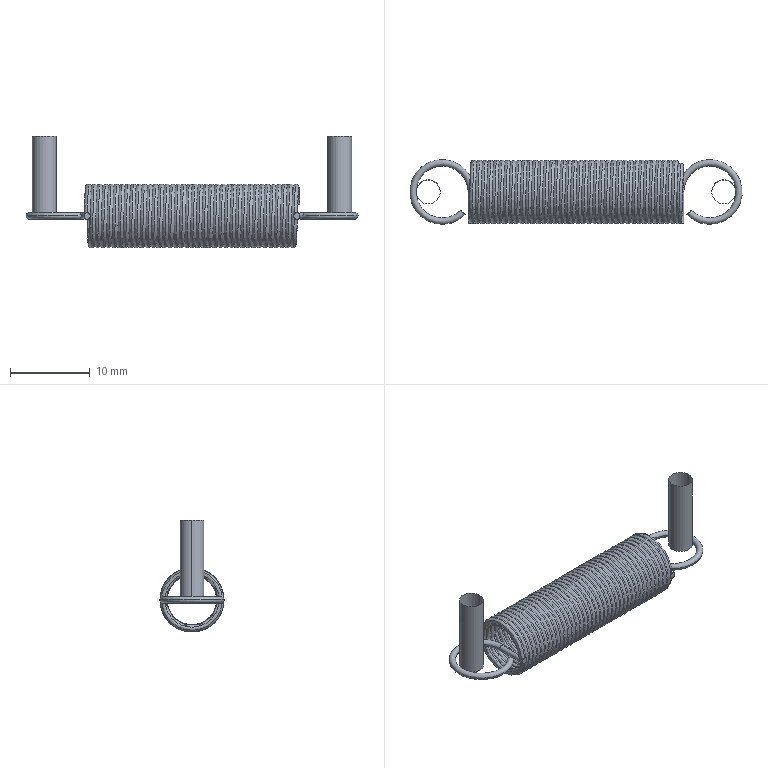Part | NX | features BREP 3 | 1 solid | 27 faces | box 41.6 x 8.1 x 14 mm | volume 518.978 mm3 | cylinder 9 | spline 9 | plane 5 | torus 4 | commonest cylinder face diameters 0.8 x5 3 x4